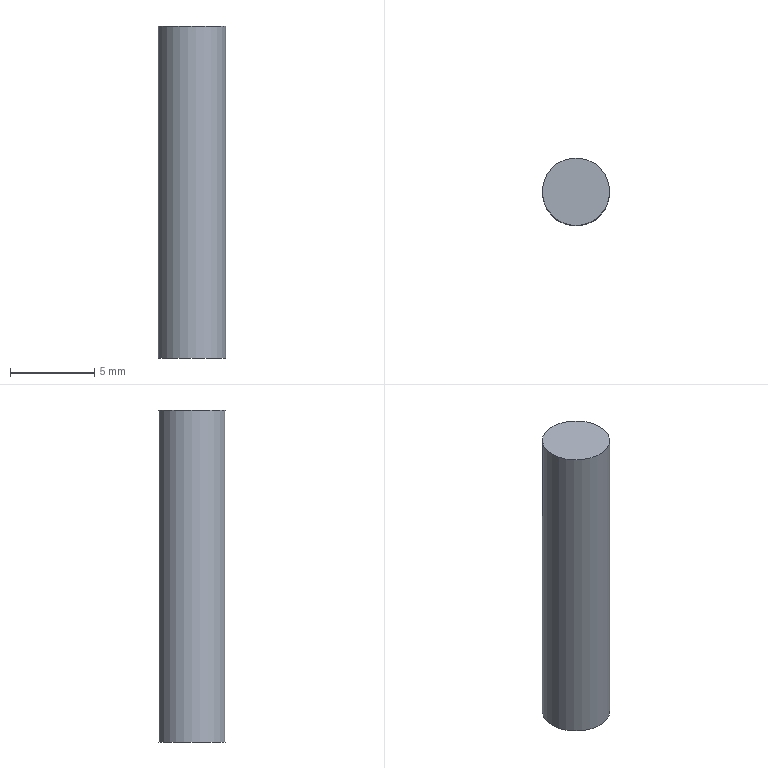Part | NX | features solid 2 | 1 solid | 3 faces | box 4 x 4 x 19.708 mm | volume 247.654 mm3 | plane 2 | cylinder 1 | commonest cylinder face diameters 4 x1
STEP:
#1=CARTESIAN_POINT('',(281.143,-474.5,67.));
#2=VERTEX_POINT('',#1);
#3=CARTESIAN_POINT('',(279.143,-474.5,67.));
#4=DIRECTION('',(0.,0.,1.));
#5=DIRECTION('',(1.,0.,0.));
#6=AXIS2_PLACEMENT_3D('',#3,#4,#5);
#7=CIRCLE('',#6,2.);
#8=EDGE_CURVE('',#2,#2,#7,.T.);
#9=ORIENTED_EDGE('',*,*,#8,.T.);
#10=EDGE_LOOP('',(#9));
#11=FACE_BOUND('',#10,.T.);
#12=CARTESIAN_POINT('',(281.143,-474.5,86.708));
#13=VERTEX_POINT('',#12);
#14=CARTESIAN_POINT('',(279.143,-474.5,86.708));
#15=DIRECTION('',(0.,0.,1.));
#16=DIRECTION('',(1.,0.,0.));
#17=AXIS2_PLACEMENT_3D('',#14,#15,#16);
#18=CIRCLE('',#17,2.);
#19=EDGE_CURVE('',#13,#13,#18,.F.);
#20=ORIENTED_EDGE('',*,*,#19,.T.);
#21=EDGE_LOOP('',(#20));
#22=FACE_BOUND('',#21,.T.);
#23=CARTESIAN_POINT('',(279.143,-474.5,67.));
#24=DIRECTION('',(0.,0.,1.));
#25=DIRECTION('',(1.,0.,0.));
#26=AXIS2_PLACEMENT_3D('',#23,#24,#25);
#27=CYLINDRICAL_SURFACE('',#26,2.);
#28=ADVANCED_FACE('',(#11,#22),#27,.T.);
#29=ORIENTED_EDGE('',*,*,#8,.F.);
#30=EDGE_LOOP('',(#29));
#31=FACE_BOUND('',#30,.T.);
#32=CARTESIAN_POINT('',(279.143,-474.5,67.));
#33=DIRECTION('',(0.,0.,-1.));
#34=DIRECTION('',(-1.,0.,0.));
#35=AXIS2_PLACEMENT_3D('',#32,#33,#34);
#36=PLANE('',#35);
#37=ADVANCED_FACE('',(#31),#36,.T.);
#38=ORIENTED_EDGE('',*,*,#19,.F.);
#39=EDGE_LOOP('',(#38));
#40=FACE_BOUND('',#39,.T.);
#41=CARTESIAN_POINT('',(426.488,227.578,86.708));
#42=DIRECTION('',(0.,0.,1.));
#43=DIRECTION('',(0.,-1.,0.));
#44=AXIS2_PLACEMENT_3D('',#41,#42,#43);
#45=PLANE('',#44);
#46=ADVANCED_FACE('',(#40),#45,.T.);
#47=CLOSED_SHELL('',(#28,#37,#46));
#48=MANIFOLD_SOLID_BREP('',#47);
#49=(LENGTH_UNIT()NAMED_UNIT(*)SI_UNIT(.MILLI.,.METRE.));
#50=UNCERTAINTY_MEASURE_WITH_UNIT(LENGTH_MEASURE(0.00001),#49,'','');
#51=(NAMED_UNIT(*)PLANE_ANGLE_UNIT()SI_UNIT($,.RADIAN.));
#52=(NAMED_UNIT(*)SI_UNIT($,.STERADIAN.)SOLID_ANGLE_UNIT());
#53=(GEOMETRIC_REPRESENTATION_CONTEXT(3)GLOBAL_UNCERTAINTY_ASSIGNED_CONTEXT((#50))GLOBAL_UNIT_ASSIGNED_CONTEXT((#49,#51,#52))REPRESENTATION_CONTEXT('',''));
#54=ADVANCED_BREP_SHAPE_REPRESENTATION('',(#48),#53);